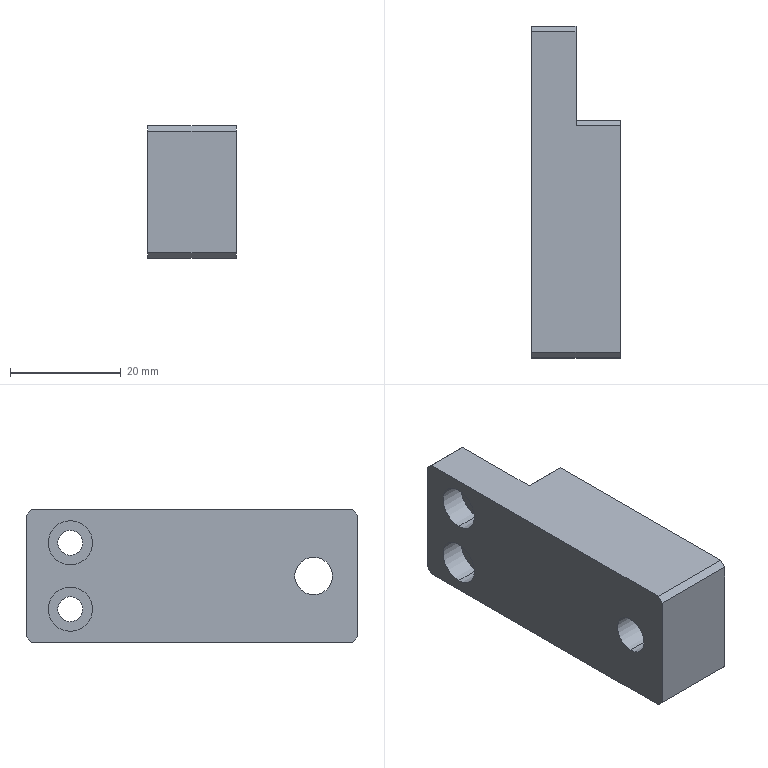Part | SolidWorks | features BaseBody 1, Chamfer 1, HoleWzd 1, ICE 1 | 1 solid | 26 faces | box 16 x 60 x 24 mm | volume 18592 mm3 | plane 16 | cylinder 10 | commonest cylinder face diameters 4.5 x4 8 x4 6.8 x2
STEP:
#1=CARTESIAN_POINT('',(0.,-22.,15.4));
#2=VERTEX_POINT('',#1);
#3=CARTESIAN_POINT('',(0.,-22.,8.6));
#4=VERTEX_POINT('',#3);
#5=CARTESIAN_POINT('',(0.,-22.,12.));
#6=DIRECTION('',(1.,0.,0.));
#7=DIRECTION('',(0.,0.,-1.));
#8=AXIS2_PLACEMENT_3D('',#5,#6,#7);
#9=CIRCLE('',#8,3.4);
#10=EDGE_CURVE('',#2,#4,#9,.T.);
#11=ORIENTED_EDGE('',*,*,#10,.F.);
#12=CARTESIAN_POINT('',(16.,-22.,15.4));
#13=VERTEX_POINT('',#12);
#14=CARTESIAN_POINT('',(16.,-22.,15.4));
#15=DIRECTION('',(1.,0.,0.));
#16=VECTOR('',#15,1000.);
#17=LINE('',#14,#16);
#18=EDGE_CURVE('',#2,#13,#17,.T.);
#19=ORIENTED_EDGE('',*,*,#18,.T.);
#20=CARTESIAN_POINT('',(16.,-22.,8.6));
#21=VERTEX_POINT('',#20);
#22=CARTESIAN_POINT('',(16.,-22.,12.));
#23=DIRECTION('',(1.,0.,0.));
#24=DIRECTION('',(0.,0.,-1.));
#25=AXIS2_PLACEMENT_3D('',#22,#23,#24);
#26=CIRCLE('',#25,3.4);
#27=EDGE_CURVE('',#13,#21,#26,.T.);
#28=ORIENTED_EDGE('',*,*,#27,.T.);
#29=CARTESIAN_POINT('',(16.,-22.,8.6));
#30=DIRECTION('',(1.,0.,0.));
#31=VECTOR('',#30,1000.);
#32=LINE('',#29,#31);
#33=EDGE_CURVE('',#4,#21,#32,.T.);
#34=ORIENTED_EDGE('',*,*,#33,.F.);
#35=EDGE_LOOP('',(#11,#19,#28,#34));
#36=FACE_OUTER_BOUND('',#35,.T.);
#37=CARTESIAN_POINT('',(16.,-22.,12.));
#38=DIRECTION('',(1.,0.,0.));
#39=DIRECTION('',(0.,0.,-1.));
#40=AXIS2_PLACEMENT_3D('',#37,#38,#39);
#41=CYLINDRICAL_SURFACE('',#40,3.4);
#42=ADVANCED_FACE('',(#36),#41,.F.);
#43=CARTESIAN_POINT('',(4.6,22.,2.));
#44=VERTEX_POINT('',#43);
#45=CARTESIAN_POINT('',(4.6,22.,10.));
#46=VERTEX_POINT('',#45);
#47=CARTESIAN_POINT('',(4.6,22.,6.));
#48=DIRECTION('',(-1.,0.,0.));
#49=DIRECTION('',(0.,0.,1.));
#50=AXIS2_PLACEMENT_3D('',#47,#48,#49);
#51=CIRCLE('',#50,4.);
#52=EDGE_CURVE('',#44,#46,#51,.T.);
#53=ORIENTED_EDGE('',*,*,#52,.F.);
#54=CARTESIAN_POINT('',(0.,22.,2.));
#55=VERTEX_POINT('',#54);
#56=CARTESIAN_POINT('',(0.,22.,2.));
#57=DIRECTION('',(-1.,0.,0.));
#58=VECTOR('',#57,1000.);
#59=LINE('',#56,#58);
#60=EDGE_CURVE('',#44,#55,#59,.T.);
#61=ORIENTED_EDGE('',*,*,#60,.T.);
#62=CARTESIAN_POINT('',(0.,22.,10.));
#63=VERTEX_POINT('',#62);
#64=CARTESIAN_POINT('',(0.,22.,6.));
#65=DIRECTION('',(-1.,0.,0.));
#66=DIRECTION('',(0.,0.,1.));
#67=AXIS2_PLACEMENT_3D('',#64,#65,#66);
#68=CIRCLE('',#67,4.);
#69=EDGE_CURVE('',#55,#63,#68,.T.);
#70=ORIENTED_EDGE('',*,*,#69,.T.);
#71=CARTESIAN_POINT('',(0.,22.,10.));
#72=DIRECTION('',(-1.,0.,0.));
#73=VECTOR('',#72,1000.);
#74=LINE('',#71,#73);
#75=EDGE_CURVE('',#46,#63,#74,.T.);
#76=ORIENTED_EDGE('',*,*,#75,.F.);
#77=EDGE_LOOP('',(#53,#61,#70,#76));
#78=FACE_OUTER_BOUND('',#77,.T.);
#79=CARTESIAN_POINT('',(0.,22.,6.));
#80=DIRECTION('',(-1.,0.,0.));
#81=DIRECTION('',(0.,0.,1.));
#82=AXIS2_PLACEMENT_3D('',#79,#80,#81);
#83=CYLINDRICAL_SURFACE('',#82,4.);
#84=ADVANCED_FACE('',(#78),#83,.F.);
#85=CARTESIAN_POINT('',(8.,22.,3.75));
#86=VERTEX_POINT('',#85);
#87=CARTESIAN_POINT('',(8.,22.,8.25));
#88=VERTEX_POINT('',#87);
#89=CARTESIAN_POINT('',(8.,22.,6.));
#90=DIRECTION('',(-1.,0.,0.));
#91=DIRECTION('',(0.,-1.,0.));
#92=AXIS2_PLACEMENT_3D('',#89,#90,#91);
#93=CIRCLE('',#92,2.25);
#94=EDGE_CURVE('',#86,#88,#93,.T.);
#95=ORIENTED_EDGE('',*,*,#94,.F.);
#96=CARTESIAN_POINT('',(4.6,22.,3.75));
#97=VERTEX_POINT('',#96);
#98=CARTESIAN_POINT('',(0.,22.,3.75));
#99=DIRECTION('',(-1.,0.,0.));
#100=VECTOR('',#99,1000.);
#101=LINE('',#98,#100);
#102=EDGE_CURVE('',#86,#97,#101,.T.);
#103=ORIENTED_EDGE('',*,*,#102,.T.);
#104=CARTESIAN_POINT('',(4.6,22.,8.25));
#105=VERTEX_POINT('',#104);
#106=CARTESIAN_POINT('',(4.6,22.,6.));
#107=DIRECTION('',(-1.,0.,0.));
#108=DIRECTION('',(0.,0.,1.));
#109=AXIS2_PLACEMENT_3D('',#106,#107,#108);
#110=CIRCLE('',#109,2.25);
#111=EDGE_CURVE('',#97,#105,#110,.T.);
#112=ORIENTED_EDGE('',*,*,#111,.T.);
#113=CARTESIAN_POINT('',(0.,22.,8.25));
#114=DIRECTION('',(-1.,0.,0.));
#115=VECTOR('',#114,1000.);
#116=LINE('',#113,#115);
#117=EDGE_CURVE('',#88,#105,#116,.T.);
#118=ORIENTED_EDGE('',*,*,#117,.F.);
#119=EDGE_LOOP('',(#95,#103,#112,#118));
#120=FACE_OUTER_BOUND('',#119,.T.);
#121=CARTESIAN_POINT('',(0.,22.,6.));
#122=DIRECTION('',(-1.,0.,0.));
#123=DIRECTION('',(0.,0.,1.));
#124=AXIS2_PLACEMENT_3D('',#121,#122,#123);
#125=CYLINDRICAL_SURFACE('',#124,2.25);
#126=ADVANCED_FACE('',(#120),#125,.F.);
#127=CARTESIAN_POINT('',(4.6,22.,14.));
#128=VERTEX_POINT('',#127);
#129=CARTESIAN_POINT('',(4.6,22.,22.));
#130=VERTEX_POINT('',#129);
#131=CARTESIAN_POINT('',(4.6,22.,18.));
#132=DIRECTION('',(-1.,0.,0.));
#133=DIRECTION('',(0.,0.,1.));
#134=AXIS2_PLACEMENT_3D('',#131,#132,#133);
#135=CIRCLE('',#134,4.);
#136=EDGE_CURVE('',#128,#130,#135,.T.);
#137=ORIENTED_EDGE('',*,*,#136,.F.);
#138=CARTESIAN_POINT('',(0.,22.,14.));
#139=VERTEX_POINT('',#138);
#140=CARTESIAN_POINT('',(0.,22.,14.));
#141=DIRECTION('',(-1.,0.,0.));
#142=VECTOR('',#141,1000.);
#143=LINE('',#140,#142);
#144=EDGE_CURVE('',#128,#139,#143,.T.);
#145=ORIENTED_EDGE('',*,*,#144,.T.);
#146=CARTESIAN_POINT('',(0.,22.,22.));
#147=VERTEX_POINT('',#146);
#148=CARTESIAN_POINT('',(0.,22.,18.));
#149=DIRECTION('',(-1.,0.,0.));
#150=DIRECTION('',(0.,0.,1.));
#151=AXIS2_PLACEMENT_3D('',#148,#149,#150);
#152=CIRCLE('',#151,4.);
#153=EDGE_CURVE('',#139,#147,#152,.T.);
#154=ORIENTED_EDGE('',*,*,#153,.T.);
#155=CARTESIAN_POINT('',(0.,22.,22.));
#156=DIRECTION('',(-1.,0.,0.));
#157=VECTOR('',#156,1000.);
#158=LINE('',#155,#157);
#159=EDGE_CURVE('',#130,#147,#158,.T.);
#160=ORIENTED_EDGE('',*,*,#159,.F.);
#161=EDGE_LOOP('',(#137,#145,#154,#160));
#162=FACE_OUTER_BOUND('',#161,.T.);
#163=CARTESIAN_POINT('',(0.,22.,18.));
#164=DIRECTION('',(-1.,0.,0.));
#165=DIRECTION('',(0.,0.,1.));
#166=AXIS2_PLACEMENT_3D('',#163,#164,#165);
#167=CYLINDRICAL_SURFACE('',#166,4.);
#168=ADVANCED_FACE('',(#162),#167,.F.);
#169=CARTESIAN_POINT('',(8.,22.,15.75));
#170=VERTEX_POINT('',#169);
#171=CARTESIAN_POINT('',(8.,22.,20.25));
#172=VERTEX_POINT('',#171);
#173=CARTESIAN_POINT('',(8.,22.,18.));
#174=DIRECTION('',(-1.,0.,0.));
#175=DIRECTION('',(0.,-1.,0.));
#176=AXIS2_PLACEMENT_3D('',#173,#174,#175);
#177=CIRCLE('',#176,2.25);
#178=EDGE_CURVE('',#170,#172,#177,.T.);
#179=ORIENTED_EDGE('',*,*,#178,.F.);
#180=CARTESIAN_POINT('',(4.6,22.,15.75));
#181=VERTEX_POINT('',#180);
#182=CARTESIAN_POINT('',(0.,22.,15.75));
#183=DIRECTION('',(-1.,0.,0.));
#184=VECTOR('',#183,1000.);
#185=LINE('',#182,#184);
#186=EDGE_CURVE('',#170,#181,#185,.T.);
#187=ORIENTED_EDGE('',*,*,#186,.T.);
#188=CARTESIAN_POINT('',(4.6,22.,20.25));
#189=VERTEX_POINT('',#188);
#190=CARTESIAN_POINT('',(4.6,22.,18.));
#191=DIRECTION('',(-1.,0.,0.));
#192=DIRECTION('',(0.,0.,1.));
#193=AXIS2_PLACEMENT_3D('',#190,#191,#192);
#194=CIRCLE('',#193,2.25);
#195=EDGE_CURVE('',#181,#189,#194,.T.);
#196=ORIENTED_EDGE('',*,*,#195,.T.);
#197=CARTESIAN_POINT('',(0.,22.,20.25));
#198=DIRECTION('',(-1.,0.,0.));
#199=VECTOR('',#198,1000.);
#200=LINE('',#197,#199);
#201=EDGE_CURVE('',#172,#189,#200,.T.);
#202=ORIENTED_EDGE('',*,*,#201,.F.);
#203=EDGE_LOOP('',(#179,#187,#196,#202));
#204=FACE_OUTER_BOUND('',#203,.T.);
#205=CARTESIAN_POINT('',(0.,22.,18.));
#206=DIRECTION('',(-1.,0.,0.));
#207=DIRECTION('',(0.,0.,1.));
#208=AXIS2_PLACEMENT_3D('',#205,#206,#207);
#209=CYLINDRICAL_SURFACE('',#208,2.25);
#210=ADVANCED_FACE('',(#204),#209,.F.);
#211=CARTESIAN_POINT('',(16.,-22.,12.));
#212=DIRECTION('',(1.,0.,0.));
#213=DIRECTION('',(0.,0.,-1.));
#214=AXIS2_PLACEMENT_3D('',#211,#212,#213);
#215=CIRCLE('',#214,3.4);
#216=EDGE_CURVE('',#21,#13,#215,.T.);
#217=ORIENTED_EDGE('',*,*,#216,.F.);
#218=ORIENTED_EDGE('',*,*,#27,.F.);
#219=EDGE_LOOP('',(#217,#218));
#220=FACE_BOUND('',#219,.T.);
#221=CARTESIAN_POINT('',(16.,-29.,24.));
#222=VERTEX_POINT('',#221);
#223=CARTESIAN_POINT('',(16.,12.,24.));
#224=VERTEX_POINT('',#223);
#225=CARTESIAN_POINT('',(16.,13.,24.));
#226=DIRECTION('',(0.,1.,0.));
#227=VECTOR('',#226,1000.);
#228=LINE('',#225,#227);
#229=EDGE_CURVE('',#222,#224,#228,.T.);
#230=ORIENTED_EDGE('',*,*,#229,.F.);
#231=CARTESIAN_POINT('',(16.,-30.,23.));
#232=VERTEX_POINT('',#231);
#233=CARTESIAN_POINT('',(16.,-30.,23.));
#234=DIRECTION('',(0.,-0.7071,-0.7071));
#235=VECTOR('',#234,1000.);
#236=LINE('',#233,#235);
#237=EDGE_CURVE('',#222,#232,#236,.T.);
#238=ORIENTED_EDGE('',*,*,#237,.T.);
#239=CARTESIAN_POINT('',(16.,-30.,1.));
#240=VERTEX_POINT('',#239);
#241=CARTESIAN_POINT('',(16.,-30.,0.));
#242=DIRECTION('',(0.,0.,-1.));
#243=VECTOR('',#242,1000.);
#244=LINE('',#241,#243);
#245=EDGE_CURVE('',#232,#240,#244,.T.);
#246=ORIENTED_EDGE('',*,*,#245,.T.);
#247=CARTESIAN_POINT('',(16.,-29.,0.));
#248=VERTEX_POINT('',#247);
#249=CARTESIAN_POINT('',(16.,-29.,0.));
#250=DIRECTION('',(0.,0.7071,-0.7071));
#251=VECTOR('',#250,1000.);
#252=LINE('',#249,#251);
#253=EDGE_CURVE('',#240,#248,#252,.T.);
#254=ORIENTED_EDGE('',*,*,#253,.T.);
#255=CARTESIAN_POINT('',(16.,12.,0.));
#256=VERTEX_POINT('',#255);
#257=CARTESIAN_POINT('',(16.,13.,0.));
#258=DIRECTION('',(0.,1.,0.));
#259=VECTOR('',#258,1000.);
#260=LINE('',#257,#259);
#261=EDGE_CURVE('',#248,#256,#260,.T.);
#262=ORIENTED_EDGE('',*,*,#261,.T.);
#263=CARTESIAN_POINT('',(16.,13.,1.));
#264=VERTEX_POINT('',#263);
#265=CARTESIAN_POINT('',(16.,13.,1.));
#266=DIRECTION('',(0.,0.7071,0.7071));
#267=VECTOR('',#266,1000.);
#268=LINE('',#265,#267);
#269=EDGE_CURVE('',#256,#264,#268,.T.);
#270=ORIENTED_EDGE('',*,*,#269,.T.);
#271=CARTESIAN_POINT('',(16.,13.,23.));
#272=VERTEX_POINT('',#271);
#273=CARTESIAN_POINT('',(16.,13.,24.));
#274=DIRECTION('',(0.,0.,-1.));
#275=VECTOR('',#274,1000.);
#276=LINE('',#273,#275);
#277=EDGE_CURVE('',#272,#264,#276,.T.);
#278=ORIENTED_EDGE('',*,*,#277,.F.);
#279=CARTESIAN_POINT('',(16.,12.,24.));
#280=DIRECTION('',(0.,-0.7071,0.7071));
#281=VECTOR('',#280,1000.);
#282=LINE('',#279,#281);
#283=EDGE_CURVE('',#272,#224,#282,.T.);
#284=ORIENTED_EDGE('',*,*,#283,.T.);
#285=EDGE_LOOP('',(#230,#238,#246,#254,#262,#270,#278,#284));
#286=FACE_OUTER_BOUND('',#285,.T.);
#287=CARTESIAN_POINT('',(16.,13.,24.));
#288=DIRECTION('',(-1.,0.,0.));
#289=DIRECTION('',(0.,0.,1.));
#290=AXIS2_PLACEMENT_3D('',#287,#288,#289);
#291=PLANE('',#290);
#292=ADVANCED_FACE('',(#220,#286),#291,.F.);
#293=CARTESIAN_POINT('',(8.,13.,23.));
#294=VERTEX_POINT('',#293);
#295=CARTESIAN_POINT('',(8.,13.,1.));
#296=VERTEX_POINT('',#295);
#297=CARTESIAN_POINT('',(8.,13.,24.));
#298=DIRECTION('',(0.,0.,-1.));
#299=VECTOR('',#298,1000.);
#300=LINE('',#297,#299);
#301=EDGE_CURVE('',#294,#296,#300,.T.);
#302=ORIENTED_EDGE('',*,*,#301,.F.);
#303=CARTESIAN_POINT('',(8.,13.,23.));
#304=DIRECTION('',(1.,0.,0.));
#305=VECTOR('',#304,1000.);
#306=LINE('',#303,#305);
#307=EDGE_CURVE('',#294,#272,#306,.T.);
#308=ORIENTED_EDGE('',*,*,#307,.T.);
#309=ORIENTED_EDGE('',*,*,#277,.T.);
#310=CARTESIAN_POINT('',(8.,13.,1.));
#311=DIRECTION('',(-1.,0.,0.));
#312=VECTOR('',#311,1000.);
#313=LINE('',#310,#312);
#314=EDGE_CURVE('',#264,#296,#313,.T.);
#315=ORIENTED_EDGE('',*,*,#314,.T.);
#316=EDGE_LOOP('',(#302,#308,#309,#315));
#317=FACE_OUTER_BOUND('',#316,.T.);
#318=CARTESIAN_POINT('',(8.,13.,24.));
#319=DIRECTION('',(0.,-1.,0.));
#320=DIRECTION('',(0.,0.,-1.));
#321=AXIS2_PLACEMENT_3D('',#318,#319,#320);
#322=PLANE('',#321);
#323=ADVANCED_FACE('',(#317),#322,.F.);
#324=CARTESIAN_POINT('',(8.,22.,6.));
#325=DIRECTION('',(-1.,0.,0.));
#326=DIRECTION('',(0.,-1.,0.));
#327=AXIS2_PLACEMENT_3D('',#324,#325,#326);
#328=CIRCLE('',#327,2.25);
#329=EDGE_CURVE('',#88,#86,#328,.T.);
#330=ORIENTED_EDGE('',*,*,#329,.T.);
#331=ORIENTED_EDGE('',*,*,#94,.T.);
#332=EDGE_LOOP('',(#330,#331));
#333=FACE_BOUND('',#332,.T.);
#334=CARTESIAN_POINT('',(8.,22.,18.));
#335=DIRECTION('',(-1.,0.,0.));
#336=DIRECTION('',(0.,-1.,0.));
#337=AXIS2_PLACEMENT_3D('',#334,#335,#336);
#338=CIRCLE('',#337,2.25);
#339=EDGE_CURVE('',#172,#170,#338,.T.);
#340=ORIENTED_EDGE('',*,*,#339,.T.);
#341=ORIENTED_EDGE('',*,*,#178,.T.);
#342=EDGE_LOOP('',(#340,#341));
#343=FACE_BOUND('',#342,.T.);
#344=CARTESIAN_POINT('',(8.,12.,0.));
#345=VERTEX_POINT('',#344);
#346=CARTESIAN_POINT('',(8.,29.,0.));
#347=VERTEX_POINT('',#346);
#348=CARTESIAN_POINT('',(8.,30.,0.));
#349=DIRECTION('',(0.,1.,0.));
#350=VECTOR('',#349,1000.);
#351=LINE('',#348,#350);
#352=EDGE_CURVE('',#345,#347,#351,.T.);
#353=ORIENTED_EDGE('',*,*,#352,.T.);
#354=CARTESIAN_POINT('',(8.,30.,1.));
#355=VERTEX_POINT('',#354);
#356=CARTESIAN_POINT('',(8.,30.,1.));
#357=DIRECTION('',(0.,0.7071,0.7071));
#358=VECTOR('',#357,1000.);
#359=LINE('',#356,#358);
#360=EDGE_CURVE('',#347,#355,#359,.T.);
#361=ORIENTED_EDGE('',*,*,#360,.T.);
#362=CARTESIAN_POINT('',(8.,30.,23.));
#363=VERTEX_POINT('',#362);
#364=CARTESIAN_POINT('',(8.,30.,24.));
#365=DIRECTION('',(0.,0.,-1.));
#366=VECTOR('',#365,1000.);
#367=LINE('',#364,#366);
#368=EDGE_CURVE('',#363,#355,#367,.T.);
#369=ORIENTED_EDGE('',*,*,#368,.F.);
#370=CARTESIAN_POINT('',(8.,29.,24.));
#371=VERTEX_POINT('',#370);
#372=CARTESIAN_POINT('',(8.,29.,24.));
#373=DIRECTION('',(0.,-0.7071,0.7071));
#374=VECTOR('',#373,1000.);
#375=LINE('',#372,#374);
#376=EDGE_CURVE('',#363,#371,#375,.T.);
#377=ORIENTED_EDGE('',*,*,#376,.T.);
#378=CARTESIAN_POINT('',(8.,12.,24.));
#379=VERTEX_POINT('',#378);
#380=CARTESIAN_POINT('',(8.,30.,24.));
#381=DIRECTION('',(0.,1.,0.));
#382=VECTOR('',#381,1000.);
#383=LINE('',#380,#382);
#384=EDGE_CURVE('',#379,#371,#383,.T.);
#385=ORIENTED_EDGE('',*,*,#384,.F.);
#386=CARTESIAN_POINT('',(8.,21.,15.));
#387=DIRECTION('',(0.,0.7071,-0.7071));
#388=VECTOR('',#387,1000.);
#389=LINE('',#386,#388);
#390=EDGE_CURVE('',#379,#294,#389,.T.);
#391=ORIENTED_EDGE('',*,*,#390,.T.);
#392=ORIENTED_EDGE('',*,*,#301,.T.);
#393=CARTESIAN_POINT('',(8.,33.,21.));
#394=DIRECTION('',(0.,-0.7071,-0.7071));
#395=VECTOR('',#394,1000.);
#396=LINE('',#393,#395);
#397=EDGE_CURVE('',#296,#345,#396,.T.);
#398=ORIENTED_EDGE('',*,*,#397,.T.);
#399=EDGE_LOOP('',(#353,#361,#369,#377,#385,#391,#392,#398));
#400=FACE_OUTER_BOUND('',#399,.T.);
#401=CARTESIAN_POINT('',(8.,30.,24.));
#402=DIRECTION('',(-1.,0.,0.));
#403=DIRECTION('',(0.,-1.,0.));
#404=AXIS2_PLACEMENT_3D('',#401,#402,#403);
#405=PLANE('',#404);
#406=ADVANCED_FACE('',(#333,#343,#400),#405,.F.);
#407=ORIENTED_EDGE('',*,*,#368,.T.);
#408=CARTESIAN_POINT('',(0.,30.,1.));
#409=VERTEX_POINT('',#408);
#410=CARTESIAN_POINT('',(0.,30.,1.));
#411=DIRECTION('',(-1.,0.,0.));
#412=VECTOR('',#411,1000.);
#413=LINE('',#410,#412);
#414=EDGE_CURVE('',#355,#409,#413,.T.);
#415=ORIENTED_EDGE('',*,*,#414,.T.);
#416=CARTESIAN_POINT('',(0.,30.,23.));
#417=VERTEX_POINT('',#416);
#418=CARTESIAN_POINT('',(0.,30.,24.));
#419=DIRECTION('',(0.,0.,-1.));
#420=VECTOR('',#419,1000.);
#421=LINE('',#418,#420);
#422=EDGE_CURVE('',#417,#409,#421,.T.);
#423=ORIENTED_EDGE('',*,*,#422,.F.);
#424=CARTESIAN_POINT('',(0.,30.,23.));
#425=DIRECTION('',(1.,0.,0.));
#426=VECTOR('',#425,1000.);
#427=LINE('',#424,#426);
#428=EDGE_CURVE('',#417,#363,#427,.T.);
#429=ORIENTED_EDGE('',*,*,#428,.T.);
#430=EDGE_LOOP('',(#407,#415,#423,#429));
#431=FACE_OUTER_BOUND('',#430,.T.);
#432=CARTESIAN_POINT('',(0.,30.,24.));
#433=DIRECTION('',(0.,-1.,0.));
#434=DIRECTION('',(0.,0.,-1.));
#435=AXIS2_PLACEMENT_3D('',#432,#433,#434);
#436=PLANE('',#435);
#437=ADVANCED_FACE('',(#431),#436,.F.);
#438=CARTESIAN_POINT('',(0.,-22.,12.));
#439=DIRECTION('',(1.,0.,0.));
#440=DIRECTION('',(0.,0.,-1.));
#441=AXIS2_PLACEMENT_3D('',#438,#439,#440);
#442=CIRCLE('',#441,3.4);
#443=EDGE_CURVE('',#4,#2,#442,.T.);
#444=ORIENTED_EDGE('',*,*,#443,.T.);
#445=ORIENTED_EDGE('',*,*,#10,.T.);
#446=EDGE_LOOP('',(#444,#445));
#447=FACE_BOUND('',#446,.T.);
#448=CARTESIAN_POINT('',(0.,22.,6.));
#449=DIRECTION('',(-1.,0.,0.));
#450=DIRECTION('',(0.,0.,1.));
#451=AXIS2_PLACEMENT_3D('',#448,#449,#450);
#452=CIRCLE('',#451,4.);
#453=EDGE_CURVE('',#63,#55,#452,.T.);
#454=ORIENTED_EDGE('',*,*,#453,.F.);
#455=ORIENTED_EDGE('',*,*,#69,.F.);
#456=EDGE_LOOP('',(#454,#455));
#457=FACE_BOUND('',#456,.T.);
#458=CARTESIAN_POINT('',(0.,22.,18.));
#459=DIRECTION('',(-1.,0.,0.));
#460=DIRECTION('',(0.,0.,1.));
#461=AXIS2_PLACEMENT_3D('',#458,#459,#460);
#462=CIRCLE('',#461,4.);
#463=EDGE_CURVE('',#147,#139,#462,.T.);
#464=ORIENTED_EDGE('',*,*,#463,.F.);
#465=ORIENTED_EDGE('',*,*,#153,.F.);
#466=EDGE_LOOP('',(#464,#465));
#467=FACE_BOUND('',#466,.T.);
#468=CARTESIAN_POINT('',(0.,-30.,1.));
#469=VERTEX_POINT('',#468);
#470=CARTESIAN_POINT('',(0.,-30.,23.));
#471=VERTEX_POINT('',#470);
#472=CARTESIAN_POINT('',(0.,-30.,0.));
#473=DIRECTION('',(0.,0.,1.));
#474=VECTOR('',#473,1000.);
#475=LINE('',#472,#474);
#476=EDGE_CURVE('',#469,#471,#475,.T.);
#477=ORIENTED_EDGE('',*,*,#476,.T.);
#478=CARTESIAN_POINT('',(0.,-29.,24.));
#479=VERTEX_POINT('',#478);
#480=CARTESIAN_POINT('',(0.,-30.,23.));
#481=DIRECTION('',(0.,0.7071,0.7071));
#482=VECTOR('',#481,1000.);
#483=LINE('',#480,#482);
#484=EDGE_CURVE('',#471,#479,#483,.T.);
#485=ORIENTED_EDGE('',*,*,#484,.T.);
#486=CARTESIAN_POINT('',(0.,29.,24.));
#487=VERTEX_POINT('',#486);
#488=CARTESIAN_POINT('',(0.,0.,24.));
#489=DIRECTION('',(0.,-1.,0.));
#490=VECTOR('',#489,1000.);
#491=LINE('',#488,#490);
#492=EDGE_CURVE('',#487,#479,#491,.T.);
#493=ORIENTED_EDGE('',*,*,#492,.F.);
#494=CARTESIAN_POINT('',(0.,29.,24.));
#495=DIRECTION('',(0.,0.7071,-0.7071));
#496=VECTOR('',#495,1000.);
#497=LINE('',#494,#496);
#498=EDGE_CURVE('',#487,#417,#497,.T.);
#499=ORIENTED_EDGE('',*,*,#498,.T.);
#500=ORIENTED_EDGE('',*,*,#422,.T.);
#501=CARTESIAN_POINT('',(0.,29.,0.));
#502=VERTEX_POINT('',#501);
#503=CARTESIAN_POINT('',(0.,30.,1.));
#504=DIRECTION('',(0.,-0.7071,-0.7071));
#505=VECTOR('',#504,1000.);
#506=LINE('',#503,#505);
#507=EDGE_CURVE('',#409,#502,#506,.T.);
#508=ORIENTED_EDGE('',*,*,#507,.T.);
#509=CARTESIAN_POINT('',(0.,-29.,0.));
#510=VERTEX_POINT('',#509);
#511=CARTESIAN_POINT('',(0.,0.,0.));
#512=DIRECTION('',(0.,-1.,0.));
#513=VECTOR('',#512,1000.);
#514=LINE('',#511,#513);
#515=EDGE_CURVE('',#502,#510,#514,.T.);
#516=ORIENTED_EDGE('',*,*,#515,.T.);
#517=CARTESIAN_POINT('',(0.,-29.,0.));
#518=DIRECTION('',(0.,-0.7071,0.7071));
#519=VECTOR('',#518,1000.);
#520=LINE('',#517,#519);
#521=EDGE_CURVE('',#510,#469,#520,.T.);
#522=ORIENTED_EDGE('',*,*,#521,.T.);
#523=EDGE_LOOP('',(#477,#485,#493,#499,#500,#508,#516,#522));
#524=FACE_OUTER_BOUND('',#523,.T.);
#525=CARTESIAN_POINT('',(0.,0.,24.));
#526=DIRECTION('',(1.,0.,0.));
#527=DIRECTION('',(0.,0.,-1.));
#528=AXIS2_PLACEMENT_3D('',#525,#526,#527);
#529=PLANE('',#528);
#530=ADVANCED_FACE('',(#447,#457,#467,#524),#529,.F.);
#531=ORIENTED_EDGE('',*,*,#492,.T.);
#532=CARTESIAN_POINT('',(16.,-29.,24.));
#533=DIRECTION('',(1.,0.,0.));
#534=VECTOR('',#533,1000.);
#535=LINE('',#532,#534);
#536=EDGE_CURVE('',#479,#222,#535,.T.);
#537=ORIENTED_EDGE('',*,*,#536,.T.);
#538=ORIENTED_EDGE('',*,*,#229,.T.);
#539=CARTESIAN_POINT('',(0.,12.,24.));
#540=DIRECTION('',(-1.,0.,0.));
#541=VECTOR('',#540,1000.);
#542=LINE('',#539,#541);
#543=EDGE_CURVE('',#224,#379,#542,.T.);
#544=ORIENTED_EDGE('',*,*,#543,.T.);
#545=ORIENTED_EDGE('',*,*,#384,.T.);
#546=CARTESIAN_POINT('',(0.,29.,24.));
#547=DIRECTION('',(-1.,0.,0.));
#548=VECTOR('',#547,1000.);
#549=LINE('',#546,#548);
#550=EDGE_CURVE('',#371,#487,#549,.T.);
#551=ORIENTED_EDGE('',*,*,#550,.T.);
#552=EDGE_LOOP('',(#531,#537,#538,#544,#545,#551));
#553=FACE_OUTER_BOUND('',#552,.T.);
#554=CARTESIAN_POINT('',(0.,0.,24.));
#555=DIRECTION('',(0.,0.,-1.));
#556=DIRECTION('',(-1.,0.,0.));
#557=AXIS2_PLACEMENT_3D('',#554,#555,#556);
#558=PLANE('',#557);
#559=ADVANCED_FACE('',(#553),#558,.F.);
#560=ORIENTED_EDGE('',*,*,#261,.F.);
#561=CARTESIAN_POINT('',(0.,-29.,0.));
#562=DIRECTION('',(-1.,0.,0.));
#563=VECTOR('',#562,1000.);
#564=LINE('',#561,#563);
#565=EDGE_CURVE('',#248,#510,#564,.T.);
#566=ORIENTED_EDGE('',*,*,#565,.T.);
#567=ORIENTED_EDGE('',*,*,#515,.F.);
#568=CARTESIAN_POINT('',(8.,29.,0.));
#569=DIRECTION('',(1.,0.,0.));
#570=VECTOR('',#569,1000.);
#571=LINE('',#568,#570);
#572=EDGE_CURVE('',#502,#347,#571,.T.);
#573=ORIENTED_EDGE('',*,*,#572,.T.);
#574=ORIENTED_EDGE('',*,*,#352,.F.);
#575=CARTESIAN_POINT('',(16.,12.,0.));
#576=DIRECTION('',(1.,0.,0.));
#577=VECTOR('',#576,1000.);
#578=LINE('',#575,#577);
#579=EDGE_CURVE('',#345,#256,#578,.T.);
#580=ORIENTED_EDGE('',*,*,#579,.T.);
#581=EDGE_LOOP('',(#560,#566,#567,#573,#574,#580));
#582=FACE_OUTER_BOUND('',#581,.T.);
#583=CARTESIAN_POINT('',(0.,0.,0.));
#584=DIRECTION('',(0.,0.,-1.));
#585=DIRECTION('',(-1.,0.,0.));
#586=AXIS2_PLACEMENT_3D('',#583,#584,#585);
#587=PLANE('',#586);
#588=ADVANCED_FACE('',(#582),#587,.T.);
#589=ORIENTED_EDGE('',*,*,#186,.F.);
#590=ORIENTED_EDGE('',*,*,#339,.F.);
#591=ORIENTED_EDGE('',*,*,#201,.T.);
#592=CARTESIAN_POINT('',(4.6,22.,18.));
#593=DIRECTION('',(-1.,0.,0.));
#594=DIRECTION('',(0.,0.,1.));
#595=AXIS2_PLACEMENT_3D('',#592,#593,#594);
#596=CIRCLE('',#595,2.25);
#597=EDGE_CURVE('',#189,#181,#596,.T.);
#598=ORIENTED_EDGE('',*,*,#597,.T.);
#599=EDGE_LOOP('',(#589,#590,#591,#598));
#600=FACE_OUTER_BOUND('',#599,.T.);
#601=CARTESIAN_POINT('',(0.,22.,18.));
#602=DIRECTION('',(-1.,0.,0.));
#603=DIRECTION('',(0.,0.,1.));
#604=AXIS2_PLACEMENT_3D('',#601,#602,#603);
#605=CYLINDRICAL_SURFACE('',#604,2.25);
#606=ADVANCED_FACE('',(#600),#605,.F.);
#607=ORIENTED_EDGE('',*,*,#597,.F.);
#608=ORIENTED_EDGE('',*,*,#195,.F.);
#609=EDGE_LOOP('',(#607,#608));
#610=FACE_BOUND('',#609,.T.);
#611=CARTESIAN_POINT('',(4.6,22.,18.));
#612=DIRECTION('',(-1.,0.,0.));
#613=DIRECTION('',(0.,0.,1.));
#614=AXIS2_PLACEMENT_3D('',#611,#612,#613);
#615=CIRCLE('',#614,4.);
#616=EDGE_CURVE('',#130,#128,#615,.T.);
#617=ORIENTED_EDGE('',*,*,#616,.T.);
#618=ORIENTED_EDGE('',*,*,#136,.T.);
#619=EDGE_LOOP('',(#617,#618));
#620=FACE_OUTER_BOUND('',#619,.T.);
#621=CARTESIAN_POINT('',(4.6,24.25,18.));
#622=DIRECTION('',(1.,0.,0.));
#623=DIRECTION('',(0.,0.,-1.));
#624=AXIS2_PLACEMENT_3D('',#621,#622,#623);
#625=PLANE('',#624);
#626=ADVANCED_FACE('',(#610,#620),#625,.F.);
#627=ORIENTED_EDGE('',*,*,#144,.F.);
#628=ORIENTED_EDGE('',*,*,#616,.F.);
#629=ORIENTED_EDGE('',*,*,#159,.T.);
#630=ORIENTED_EDGE('',*,*,#463,.T.);
#631=EDGE_LOOP('',(#627,#628,#629,#630));
#632=FACE_OUTER_BOUND('',#631,.T.);
#633=CARTESIAN_POINT('',(0.,22.,18.));
#634=DIRECTION('',(-1.,0.,0.));
#635=DIRECTION('',(0.,0.,1.));
#636=AXIS2_PLACEMENT_3D('',#633,#634,#635);
#637=CYLINDRICAL_SURFACE('',#636,4.);
#638=ADVANCED_FACE('',(#632),#637,.F.);
#639=ORIENTED_EDGE('',*,*,#102,.F.);
#640=ORIENTED_EDGE('',*,*,#329,.F.);
#641=ORIENTED_EDGE('',*,*,#117,.T.);
#642=CARTESIAN_POINT('',(4.6,22.,6.));
#643=DIRECTION('',(-1.,0.,0.));
#644=DIRECTION('',(0.,0.,1.));
#645=AXIS2_PLACEMENT_3D('',#642,#643,#644);
#646=CIRCLE('',#645,2.25);
#647=EDGE_CURVE('',#105,#97,#646,.T.);
#648=ORIENTED_EDGE('',*,*,#647,.T.);
#649=EDGE_LOOP('',(#639,#640,#641,#648));
#650=FACE_OUTER_BOUND('',#649,.T.);
#651=CARTESIAN_POINT('',(0.,22.,6.));
#652=DIRECTION('',(-1.,0.,0.));
#653=DIRECTION('',(0.,0.,1.));
#654=AXIS2_PLACEMENT_3D('',#651,#652,#653);
#655=CYLINDRICAL_SURFACE('',#654,2.25);
#656=ADVANCED_FACE('',(#650),#655,.F.);
#657=ORIENTED_EDGE('',*,*,#647,.F.);
#658=ORIENTED_EDGE('',*,*,#111,.F.);
#659=EDGE_LOOP('',(#657,#658));
#660=FACE_BOUND('',#659,.T.);
#661=CARTESIAN_POINT('',(4.6,22.,6.));
#662=DIRECTION('',(-1.,0.,0.));
#663=DIRECTION('',(0.,0.,1.));
#664=AXIS2_PLACEMENT_3D('',#661,#662,#663);
#665=CIRCLE('',#664,4.);
#666=EDGE_CURVE('',#46,#44,#665,.T.);
#667=ORIENTED_EDGE('',*,*,#666,.T.);
#668=ORIENTED_EDGE('',*,*,#52,.T.);
#669=EDGE_LOOP('',(#667,#668));
#670=FACE_OUTER_BOUND('',#669,.T.);
#671=CARTESIAN_POINT('',(4.6,24.25,6.));
#672=DIRECTION('',(1.,0.,0.));
#673=DIRECTION('',(0.,0.,-1.));
#674=AXIS2_PLACEMENT_3D('',#671,#672,#673);
#675=PLANE('',#674);
#676=ADVANCED_FACE('',(#660,#670),#675,.F.);
#677=ORIENTED_EDGE('',*,*,#60,.F.);
#678=ORIENTED_EDGE('',*,*,#666,.F.);
#679=ORIENTED_EDGE('',*,*,#75,.T.);
#680=ORIENTED_EDGE('',*,*,#453,.T.);
#681=EDGE_LOOP('',(#677,#678,#679,#680));
#682=FACE_OUTER_BOUND('',#681,.T.);
#683=CARTESIAN_POINT('',(0.,22.,6.));
#684=DIRECTION('',(-1.,0.,0.));
#685=DIRECTION('',(0.,0.,1.));
#686=AXIS2_PLACEMENT_3D('',#683,#684,#685);
#687=CYLINDRICAL_SURFACE('',#686,4.);
#688=ADVANCED_FACE('',(#682),#687,.F.);
#689=ORIENTED_EDGE('',*,*,#283,.F.);
#690=ORIENTED_EDGE('',*,*,#307,.F.);
#691=ORIENTED_EDGE('',*,*,#390,.F.);
#692=ORIENTED_EDGE('',*,*,#543,.F.);
#693=EDGE_LOOP('',(#689,#690,#691,#692));
#694=FACE_OUTER_BOUND('',#693,.T.);
#695=CARTESIAN_POINT('',(0.,12.,24.));
#696=DIRECTION('',(0.,-0.7071,-0.7071));
#697=DIRECTION('',(-1.,0.,0.));
#698=AXIS2_PLACEMENT_3D('',#695,#696,#697);
#699=PLANE('',#698);
#700=ADVANCED_FACE('',(#694),#699,.F.);
#701=ORIENTED_EDGE('',*,*,#269,.F.);
#702=ORIENTED_EDGE('',*,*,#579,.F.);
#703=ORIENTED_EDGE('',*,*,#397,.F.);
#704=ORIENTED_EDGE('',*,*,#314,.F.);
#705=EDGE_LOOP('',(#701,#702,#703,#704));
#706=FACE_OUTER_BOUND('',#705,.T.);
#707=CARTESIAN_POINT('',(8.,13.,1.));
#708=DIRECTION('',(0.,0.7071,-0.7071));
#709=DIRECTION('',(1.,0.,0.));
#710=AXIS2_PLACEMENT_3D('',#707,#708,#709);
#711=PLANE('',#710);
#712=ADVANCED_FACE('',(#706),#711,.T.);
#713=ORIENTED_EDGE('',*,*,#360,.F.);
#714=ORIENTED_EDGE('',*,*,#572,.F.);
#715=ORIENTED_EDGE('',*,*,#507,.F.);
#716=ORIENTED_EDGE('',*,*,#414,.F.);
#717=EDGE_LOOP('',(#713,#714,#715,#716));
#718=FACE_OUTER_BOUND('',#717,.T.);
#719=CARTESIAN_POINT('',(0.,30.,1.));
#720=DIRECTION('',(0.,0.7071,-0.7071));
#721=DIRECTION('',(1.,0.,0.));
#722=AXIS2_PLACEMENT_3D('',#719,#720,#721);
#723=PLANE('',#722);
#724=ADVANCED_FACE('',(#718),#723,.T.);
#725=ORIENTED_EDGE('',*,*,#376,.F.);
#726=ORIENTED_EDGE('',*,*,#428,.F.);
#727=ORIENTED_EDGE('',*,*,#498,.F.);
#728=ORIENTED_EDGE('',*,*,#550,.F.);
#729=EDGE_LOOP('',(#725,#726,#727,#728));
#730=FACE_OUTER_BOUND('',#729,.T.);
#731=CARTESIAN_POINT('',(0.,29.,24.));
#732=DIRECTION('',(0.,-0.7071,-0.7071));
#733=DIRECTION('',(-1.,0.,0.));
#734=AXIS2_PLACEMENT_3D('',#731,#732,#733);
#735=PLANE('',#734);
#736=ADVANCED_FACE('',(#730),#735,.F.);
#737=ORIENTED_EDGE('',*,*,#245,.F.);
#738=CARTESIAN_POINT('',(0.,-30.,23.));
#739=DIRECTION('',(-1.,0.,0.));
#740=VECTOR('',#739,1000.);
#741=LINE('',#738,#740);
#742=EDGE_CURVE('',#232,#471,#741,.T.);
#743=ORIENTED_EDGE('',*,*,#742,.T.);
#744=ORIENTED_EDGE('',*,*,#476,.F.);
#745=CARTESIAN_POINT('',(55.205,-30.,1.));
#746=DIRECTION('',(1.,0.,0.));
#747=VECTOR('',#746,1000.);
#748=LINE('',#745,#747);
#749=EDGE_CURVE('',#469,#240,#748,.T.);
#750=ORIENTED_EDGE('',*,*,#749,.T.);
#751=EDGE_LOOP('',(#737,#743,#744,#750));
#752=FACE_OUTER_BOUND('',#751,.T.);
#753=CARTESIAN_POINT('',(55.205,-30.,0.));
#754=DIRECTION('',(0.,-1.,0.));
#755=DIRECTION('',(0.,0.,-1.));
#756=AXIS2_PLACEMENT_3D('',#753,#754,#755);
#757=PLANE('',#756);
#758=ADVANCED_FACE('',(#752),#757,.T.);
#759=ORIENTED_EDGE('',*,*,#237,.F.);
#760=ORIENTED_EDGE('',*,*,#536,.F.);
#761=ORIENTED_EDGE('',*,*,#484,.F.);
#762=ORIENTED_EDGE('',*,*,#742,.F.);
#763=EDGE_LOOP('',(#759,#760,#761,#762));
#764=FACE_OUTER_BOUND('',#763,.T.);
#765=CARTESIAN_POINT('',(55.205,-30.,23.));
#766=DIRECTION('',(0.,-0.7071,0.7071));
#767=DIRECTION('',(1.,0.,0.));
#768=AXIS2_PLACEMENT_3D('',#765,#766,#767);
#769=PLANE('',#768);
#770=ADVANCED_FACE('',(#764),#769,.T.);
#771=ORIENTED_EDGE('',*,*,#253,.F.);
#772=ORIENTED_EDGE('',*,*,#749,.F.);
#773=ORIENTED_EDGE('',*,*,#521,.F.);
#774=ORIENTED_EDGE('',*,*,#565,.F.);
#775=EDGE_LOOP('',(#771,#772,#773,#774));
#776=FACE_OUTER_BOUND('',#775,.T.);
#777=CARTESIAN_POINT('',(0.,-29.,0.));
#778=DIRECTION('',(0.,0.7071,0.7071));
#779=DIRECTION('',(-1.,0.,0.));
#780=AXIS2_PLACEMENT_3D('',#777,#778,#779);
#781=PLANE('',#780);
#782=ADVANCED_FACE('',(#776),#781,.F.);
#783=ORIENTED_EDGE('',*,*,#18,.F.);
#784=ORIENTED_EDGE('',*,*,#443,.F.);
#785=ORIENTED_EDGE('',*,*,#33,.T.);
#786=ORIENTED_EDGE('',*,*,#216,.T.);
#787=EDGE_LOOP('',(#783,#784,#785,#786));
#788=FACE_OUTER_BOUND('',#787,.T.);
#789=CARTESIAN_POINT('',(16.,-22.,12.));
#790=DIRECTION('',(1.,0.,0.));
#791=DIRECTION('',(0.,0.,-1.));
#792=AXIS2_PLACEMENT_3D('',#789,#790,#791);
#793=CYLINDRICAL_SURFACE('',#792,3.4);
#794=ADVANCED_FACE('',(#788),#793,.F.);
#795=CLOSED_SHELL('',(#42,#84,#126,#168,#210,#292,#323,#406,#437,#530,#559,#588,#606,#626,#638,#656,#676,#688,#700,#712,#724,#736,#758,#770,#782,#794));
#796=MANIFOLD_SOLID_BREP('',#795);
#797=CARTESIAN_POINT('',(0.,0.,0.));
#798=DIRECTION('',(0.,0.,1.));
#799=DIRECTION('',(1.,0.,0.));
#800=AXIS2_PLACEMENT_3D('',#797,#798,#799);
#801=(LENGTH_UNIT()NAMED_UNIT(*)SI_UNIT(.MILLI.,.METRE.));
#802=UNCERTAINTY_MEASURE_WITH_UNIT(LENGTH_MEASURE(0.00001),#801,'','');
#803=(NAMED_UNIT(*)PLANE_ANGLE_UNIT()SI_UNIT($,.RADIAN.));
#804=(NAMED_UNIT(*)SI_UNIT($,.STERADIAN.)SOLID_ANGLE_UNIT());
#805=(GEOMETRIC_REPRESENTATION_CONTEXT(3)GLOBAL_UNCERTAINTY_ASSIGNED_CONTEXT((#802))GLOBAL_UNIT_ASSIGNED_CONTEXT((#801,#803,#804))REPRESENTATION_CONTEXT('',''));
#806=ADVANCED_BREP_SHAPE_REPRESENTATION('',(#796,#800),#805);